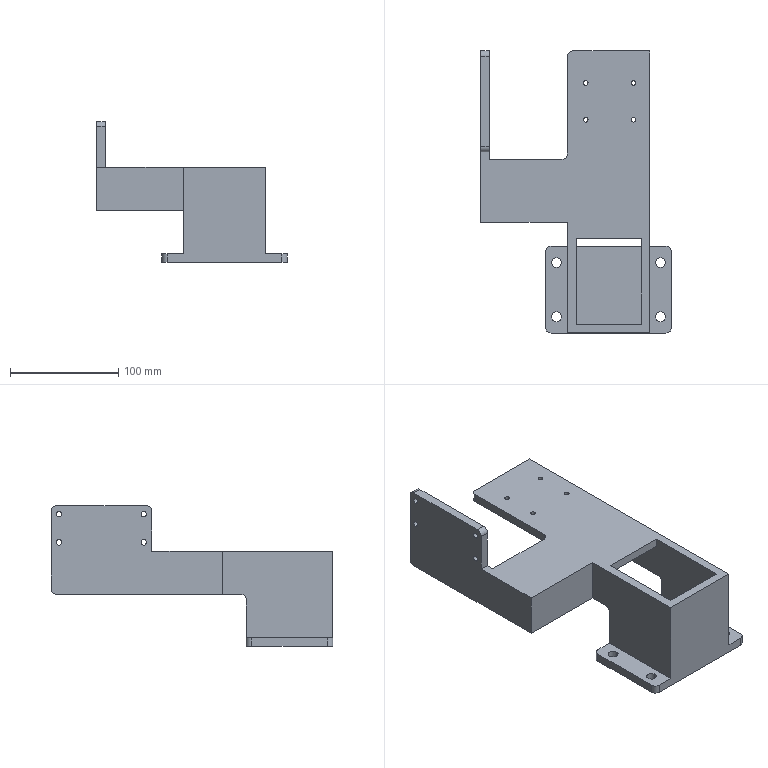Part | SolidWorks | features ICE 9, HoleWzd 4, Fillet 3, Extrusion 1, MirrorPattern 1 | 1 solid | 68 faces | box 176 x 260 x 130 mm | volume 504941 mm3 | cylinder 40 | plane 28 | commonest cylinder face diameters 4.2 x12 10 x12 5 x8 9 x8